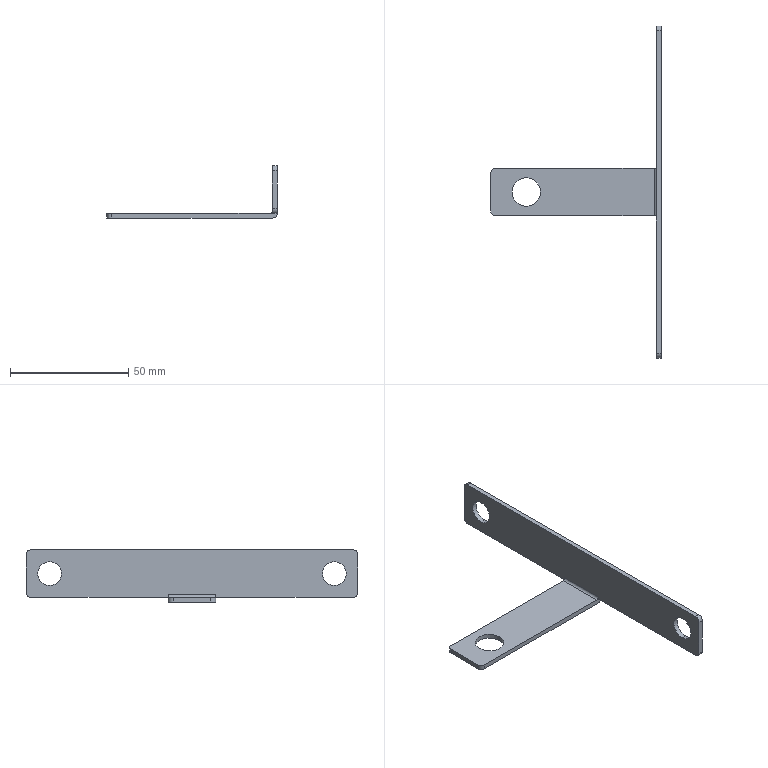Part | SolidWorks | features BaseBody 1 | 1 solid | 26 faces | box 72 x 140.21 x 22 mm | volume 7925 mm3 | cylinder 14 | plane 12 | commonest cylinder face diameters 4 x7 10 x4 12 x2 2 x1
STEP:
#1=CARTESIAN_POINT('',(0.,-10.,-9.));
#2=VERTEX_POINT('',#1);
#3=CARTESIAN_POINT('',(-1.,-10.,-10.));
#4=VERTEX_POINT('',#3);
#5=CARTESIAN_POINT('',(-1.,-10.,-9.));
#6=DIRECTION('',(0.,1.,0.));
#7=DIRECTION('',(0.,0.,1.));
#8=AXIS2_PLACEMENT_3D('',#5,#6,#7);
#9=CIRCLE('',#8,1.);
#10=EDGE_CURVE('',#2,#4,#9,.T.);
#11=ORIENTED_EDGE('',*,*,#10,.F.);
#12=CARTESIAN_POINT('',(0.,10.,-9.));
#13=VERTEX_POINT('',#12);
#14=CARTESIAN_POINT('',(0.,-10.,-9.));
#15=DIRECTION('',(0.,-1.,0.));
#16=VECTOR('',#15,1000.);
#17=LINE('',#14,#16);
#18=EDGE_CURVE('',#13,#2,#17,.T.);
#19=ORIENTED_EDGE('',*,*,#18,.F.);
#20=CARTESIAN_POINT('',(-1.,10.,-10.));
#21=VERTEX_POINT('',#20);
#22=CARTESIAN_POINT('',(-1.,10.,-9.));
#23=DIRECTION('',(0.,-1.,0.));
#24=DIRECTION('',(0.,0.,-1.));
#25=AXIS2_PLACEMENT_3D('',#22,#23,#24);
#26=CIRCLE('',#25,1.);
#27=EDGE_CURVE('',#21,#13,#26,.T.);
#28=ORIENTED_EDGE('',*,*,#27,.F.);
#29=CARTESIAN_POINT('',(-1.,10.,-10.));
#30=DIRECTION('',(0.,1.,0.));
#31=VECTOR('',#30,1000.);
#32=LINE('',#29,#31);
#33=EDGE_CURVE('',#4,#21,#32,.T.);
#34=ORIENTED_EDGE('',*,*,#33,.F.);
#35=EDGE_LOOP('',(#11,#19,#28,#34));
#36=FACE_OUTER_BOUND('',#35,.T.);
#37=CARTESIAN_POINT('',(-1.,8.,-9.));
#38=DIRECTION('',(0.,-1.,0.));
#39=DIRECTION('',(0.,0.,-1.));
#40=AXIS2_PLACEMENT_3D('',#37,#38,#39);
#41=CYLINDRICAL_SURFACE('',#40,1.);
#42=ADVANCED_FACE('',(#36),#41,.F.);
#43=CARTESIAN_POINT('',(2.,10.,-10.));
#44=VERTEX_POINT('',#43);
#45=CARTESIAN_POINT('',(0.,10.,-12.));
#46=VERTEX_POINT('',#45);
#47=CARTESIAN_POINT('',(0.,10.,-10.));
#48=DIRECTION('',(0.,1.,0.));
#49=DIRECTION('',(0.,0.,-1.));
#50=AXIS2_PLACEMENT_3D('',#47,#48,#49);
#51=CIRCLE('',#50,2.);
#52=EDGE_CURVE('',#44,#46,#51,.T.);
#53=ORIENTED_EDGE('',*,*,#52,.F.);
#54=CARTESIAN_POINT('',(2.,-10.,-10.));
#55=VERTEX_POINT('',#54);
#56=CARTESIAN_POINT('',(2.,-68.105,-10.));
#57=DIRECTION('',(0.,1.,0.));
#58=VECTOR('',#57,1000.);
#59=LINE('',#56,#58);
#60=EDGE_CURVE('',#55,#44,#59,.T.);
#61=ORIENTED_EDGE('',*,*,#60,.F.);
#62=CARTESIAN_POINT('',(0.,-10.,-12.));
#63=VERTEX_POINT('',#62);
#64=CARTESIAN_POINT('',(0.,-10.,-10.));
#65=DIRECTION('',(0.,-1.,0.));
#66=DIRECTION('',(0.,0.,1.));
#67=AXIS2_PLACEMENT_3D('',#64,#65,#66);
#68=CIRCLE('',#67,2.);
#69=EDGE_CURVE('',#63,#55,#68,.T.);
#70=ORIENTED_EDGE('',*,*,#69,.F.);
#71=CARTESIAN_POINT('',(0.,8.,-12.));
#72=DIRECTION('',(0.,-1.,0.));
#73=VECTOR('',#72,1000.);
#74=LINE('',#71,#73);
#75=EDGE_CURVE('',#46,#63,#74,.T.);
#76=ORIENTED_EDGE('',*,*,#75,.F.);
#77=EDGE_LOOP('',(#53,#61,#70,#76));
#78=FACE_OUTER_BOUND('',#77,.T.);
#79=CARTESIAN_POINT('',(0.,8.,-10.));
#80=DIRECTION('',(0.,-1.,0.));
#81=DIRECTION('',(0.,0.,-1.));
#82=AXIS2_PLACEMENT_3D('',#79,#80,#81);
#83=CYLINDRICAL_SURFACE('',#82,2.);
#84=ADVANCED_FACE('',(#78),#83,.T.);
#85=CARTESIAN_POINT('',(-61.,0.,-12.));
#86=VERTEX_POINT('',#85);
#87=CARTESIAN_POINT('',(-61.,0.,-10.));
#88=VERTEX_POINT('',#87);
#89=CARTESIAN_POINT('',(-61.,0.,-12.));
#90=DIRECTION('',(0.,0.,1.));
#91=VECTOR('',#90,1000.);
#92=LINE('',#89,#91);
#93=EDGE_CURVE('',#86,#88,#92,.T.);
#94=ORIENTED_EDGE('',*,*,#93,.F.);
#95=CARTESIAN_POINT('',(-49.,0.,-12.));
#96=VERTEX_POINT('',#95);
#97=CARTESIAN_POINT('',(-55.,0.,-12.));
#98=DIRECTION('',(0.,0.,-1.));
#99=DIRECTION('',(-1.,0.,0.));
#100=AXIS2_PLACEMENT_3D('',#97,#98,#99);
#101=CIRCLE('',#100,6.);
#102=EDGE_CURVE('',#86,#96,#101,.T.);
#103=ORIENTED_EDGE('',*,*,#102,.T.);
#104=CARTESIAN_POINT('',(-49.,0.,-10.));
#105=VERTEX_POINT('',#104);
#106=CARTESIAN_POINT('',(-49.,0.,-12.));
#107=DIRECTION('',(0.,0.,1.));
#108=VECTOR('',#107,1000.);
#109=LINE('',#106,#108);
#110=EDGE_CURVE('',#96,#105,#109,.T.);
#111=ORIENTED_EDGE('',*,*,#110,.T.);
#112=CARTESIAN_POINT('',(-55.,0.,-10.));
#113=DIRECTION('',(0.,0.,-1.));
#114=DIRECTION('',(-1.,0.,0.));
#115=AXIS2_PLACEMENT_3D('',#112,#113,#114);
#116=CIRCLE('',#115,6.);
#117=EDGE_CURVE('',#88,#105,#116,.T.);
#118=ORIENTED_EDGE('',*,*,#117,.F.);
#119=EDGE_LOOP('',(#94,#103,#111,#118));
#120=FACE_OUTER_BOUND('',#119,.T.);
#121=CARTESIAN_POINT('',(-55.,0.,-12.));
#122=DIRECTION('',(0.,0.,1.));
#123=DIRECTION('',(1.,0.,0.));
#124=AXIS2_PLACEMENT_3D('',#121,#122,#123);
#125=CYLINDRICAL_SURFACE('',#124,6.);
#126=ADVANCED_FACE('',(#120),#125,.F.);
#127=CARTESIAN_POINT('',(-70.,-8.,-10.));
#128=VERTEX_POINT('',#127);
#129=CARTESIAN_POINT('',(-70.,8.,-10.));
#130=VERTEX_POINT('',#129);
#131=CARTESIAN_POINT('',(-70.,8.,-10.));
#132=DIRECTION('',(0.,1.,0.));
#133=VECTOR('',#132,1000.);
#134=LINE('',#131,#133);
#135=EDGE_CURVE('',#128,#130,#134,.T.);
#136=ORIENTED_EDGE('',*,*,#135,.T.);
#137=CARTESIAN_POINT('',(-70.,8.,-12.));
#138=VERTEX_POINT('',#137);
#139=CARTESIAN_POINT('',(-70.,8.,-12.));
#140=DIRECTION('',(0.,0.,1.));
#141=VECTOR('',#140,1000.);
#142=LINE('',#139,#141);
#143=EDGE_CURVE('',#138,#130,#142,.T.);
#144=ORIENTED_EDGE('',*,*,#143,.F.);
#145=CARTESIAN_POINT('',(-70.,-8.,-12.));
#146=VERTEX_POINT('',#145);
#147=CARTESIAN_POINT('',(-70.,8.,-12.));
#148=DIRECTION('',(0.,1.,0.));
#149=VECTOR('',#148,1000.);
#150=LINE('',#147,#149);
#151=EDGE_CURVE('',#146,#138,#150,.T.);
#152=ORIENTED_EDGE('',*,*,#151,.F.);
#153=CARTESIAN_POINT('',(-70.,-8.,-12.));
#154=DIRECTION('',(0.,0.,1.));
#155=VECTOR('',#154,1000.);
#156=LINE('',#153,#155);
#157=EDGE_CURVE('',#146,#128,#156,.T.);
#158=ORIENTED_EDGE('',*,*,#157,.T.);
#159=EDGE_LOOP('',(#136,#144,#152,#158));
#160=FACE_OUTER_BOUND('',#159,.T.);
#161=CARTESIAN_POINT('',(-70.,8.,-12.));
#162=DIRECTION('',(1.,0.,0.));
#163=DIRECTION('',(0.,1.,0.));
#164=AXIS2_PLACEMENT_3D('',#161,#162,#163);
#165=PLANE('',#164);
#166=ADVANCED_FACE('',(#160),#165,.F.);
#167=CARTESIAN_POINT('',(-68.,-10.,-10.));
#168=VERTEX_POINT('',#167);
#169=CARTESIAN_POINT('',(-68.,-8.,-10.));
#170=DIRECTION('',(0.,0.,-1.));
#171=DIRECTION('',(1.,0.,0.));
#172=AXIS2_PLACEMENT_3D('',#169,#170,#171);
#173=CIRCLE('',#172,2.);
#174=EDGE_CURVE('',#168,#128,#173,.T.);
#175=ORIENTED_EDGE('',*,*,#174,.T.);
#176=ORIENTED_EDGE('',*,*,#157,.F.);
#177=CARTESIAN_POINT('',(-68.,-10.,-12.));
#178=VERTEX_POINT('',#177);
#179=CARTESIAN_POINT('',(-68.,-8.,-12.));
#180=DIRECTION('',(0.,0.,-1.));
#181=DIRECTION('',(1.,0.,0.));
#182=AXIS2_PLACEMENT_3D('',#179,#180,#181);
#183=CIRCLE('',#182,2.);
#184=EDGE_CURVE('',#178,#146,#183,.T.);
#185=ORIENTED_EDGE('',*,*,#184,.F.);
#186=CARTESIAN_POINT('',(-68.,-10.,-12.));
#187=DIRECTION('',(0.,0.,1.));
#188=VECTOR('',#187,1000.);
#189=LINE('',#186,#188);
#190=EDGE_CURVE('',#178,#168,#189,.T.);
#191=ORIENTED_EDGE('',*,*,#190,.T.);
#192=EDGE_LOOP('',(#175,#176,#185,#191));
#193=FACE_OUTER_BOUND('',#192,.T.);
#194=CARTESIAN_POINT('',(-68.,-8.,-12.));
#195=DIRECTION('',(0.,0.,1.));
#196=DIRECTION('',(1.,0.,0.));
#197=AXIS2_PLACEMENT_3D('',#194,#195,#196);
#198=CYLINDRICAL_SURFACE('',#197,2.);
#199=ADVANCED_FACE('',(#193),#198,.T.);
#200=CARTESIAN_POINT('',(-68.,-10.,-12.));
#201=DIRECTION('',(-1.,0.,0.));
#202=VECTOR('',#201,1000.);
#203=LINE('',#200,#202);
#204=EDGE_CURVE('',#63,#178,#203,.T.);
#205=ORIENTED_EDGE('',*,*,#204,.F.);
#206=ORIENTED_EDGE('',*,*,#69,.T.);
#207=CARTESIAN_POINT('',(0.,-10.,-10.));
#208=VERTEX_POINT('',#207);
#209=CARTESIAN_POINT('',(-68.,-10.,-10.));
#210=DIRECTION('',(-1.,0.,0.));
#211=VECTOR('',#210,1000.);
#212=LINE('',#209,#211);
#213=EDGE_CURVE('',#55,#208,#212,.T.);
#214=ORIENTED_EDGE('',*,*,#213,.T.);
#215=CARTESIAN_POINT('',(0.,-10.,-8.));
#216=DIRECTION('',(0.,0.,-1.));
#217=VECTOR('',#216,1000.);
#218=LINE('',#215,#217);
#219=EDGE_CURVE('',#2,#208,#218,.T.);
#220=ORIENTED_EDGE('',*,*,#219,.F.);
#221=ORIENTED_EDGE('',*,*,#10,.T.);
#222=CARTESIAN_POINT('',(-68.,-10.,-10.));
#223=DIRECTION('',(-1.,0.,0.));
#224=VECTOR('',#223,1000.);
#225=LINE('',#222,#224);
#226=EDGE_CURVE('',#4,#168,#225,.T.);
#227=ORIENTED_EDGE('',*,*,#226,.T.);
#228=ORIENTED_EDGE('',*,*,#190,.F.);
#229=EDGE_LOOP('',(#205,#206,#214,#220,#221,#227,#228));
#230=FACE_OUTER_BOUND('',#229,.T.);
#231=CARTESIAN_POINT('',(-68.,-10.,-12.));
#232=DIRECTION('',(0.,1.,0.));
#233=DIRECTION('',(1.,0.,0.));
#234=AXIS2_PLACEMENT_3D('',#231,#232,#233);
#235=PLANE('',#234);
#236=ADVANCED_FACE('',(#230),#235,.F.);
#237=CARTESIAN_POINT('',(0.,10.,-10.));
#238=VERTEX_POINT('',#237);
#239=CARTESIAN_POINT('',(2.,10.,-10.));
#240=DIRECTION('',(1.,0.,0.));
#241=VECTOR('',#240,1000.);
#242=LINE('',#239,#241);
#243=EDGE_CURVE('',#238,#44,#242,.T.);
#244=ORIENTED_EDGE('',*,*,#243,.T.);
#245=ORIENTED_EDGE('',*,*,#52,.T.);
#246=CARTESIAN_POINT('',(-68.,10.,-12.));
#247=VERTEX_POINT('',#246);
#248=CARTESIAN_POINT('',(2.,10.,-12.));
#249=DIRECTION('',(1.,0.,0.));
#250=VECTOR('',#249,1000.);
#251=LINE('',#248,#250);
#252=EDGE_CURVE('',#247,#46,#251,.T.);
#253=ORIENTED_EDGE('',*,*,#252,.F.);
#254=CARTESIAN_POINT('',(-68.,10.,-10.));
#255=VERTEX_POINT('',#254);
#256=CARTESIAN_POINT('',(-68.,10.,-12.));
#257=DIRECTION('',(0.,0.,1.));
#258=VECTOR('',#257,1000.);
#259=LINE('',#256,#258);
#260=EDGE_CURVE('',#247,#255,#259,.T.);
#261=ORIENTED_EDGE('',*,*,#260,.T.);
#262=CARTESIAN_POINT('',(2.,10.,-10.));
#263=DIRECTION('',(1.,0.,0.));
#264=VECTOR('',#263,1000.);
#265=LINE('',#262,#264);
#266=EDGE_CURVE('',#255,#21,#265,.T.);
#267=ORIENTED_EDGE('',*,*,#266,.T.);
#268=ORIENTED_EDGE('',*,*,#27,.T.);
#269=CARTESIAN_POINT('',(0.,10.,-8.));
#270=DIRECTION('',(0.,0.,1.));
#271=VECTOR('',#270,1000.);
#272=LINE('',#269,#271);
#273=EDGE_CURVE('',#238,#13,#272,.T.);
#274=ORIENTED_EDGE('',*,*,#273,.F.);
#275=EDGE_LOOP('',(#244,#245,#253,#261,#267,#268,#274));
#276=FACE_OUTER_BOUND('',#275,.T.);
#277=CARTESIAN_POINT('',(2.,10.,-12.));
#278=DIRECTION('',(0.,-1.,0.));
#279=DIRECTION('',(0.,0.,-1.));
#280=AXIS2_PLACEMENT_3D('',#277,#278,#279);
#281=PLANE('',#280);
#282=ADVANCED_FACE('',(#276),#281,.F.);
#283=CARTESIAN_POINT('',(-68.,8.,-10.));
#284=DIRECTION('',(0.,0.,-1.));
#285=DIRECTION('',(1.,0.,0.));
#286=AXIS2_PLACEMENT_3D('',#283,#284,#285);
#287=CIRCLE('',#286,2.);
#288=EDGE_CURVE('',#130,#255,#287,.T.);
#289=ORIENTED_EDGE('',*,*,#288,.T.);
#290=ORIENTED_EDGE('',*,*,#260,.F.);
#291=CARTESIAN_POINT('',(-68.,8.,-12.));
#292=DIRECTION('',(0.,0.,-1.));
#293=DIRECTION('',(1.,0.,0.));
#294=AXIS2_PLACEMENT_3D('',#291,#292,#293);
#295=CIRCLE('',#294,2.);
#296=EDGE_CURVE('',#138,#247,#295,.T.);
#297=ORIENTED_EDGE('',*,*,#296,.F.);
#298=ORIENTED_EDGE('',*,*,#143,.T.);
#299=EDGE_LOOP('',(#289,#290,#297,#298));
#300=FACE_OUTER_BOUND('',#299,.T.);
#301=CARTESIAN_POINT('',(-68.,8.,-12.));
#302=DIRECTION('',(0.,0.,1.));
#303=DIRECTION('',(1.,0.,0.));
#304=AXIS2_PLACEMENT_3D('',#301,#302,#303);
#305=CYLINDRICAL_SURFACE('',#304,2.);
#306=ADVANCED_FACE('',(#300),#305,.T.);
#307=CARTESIAN_POINT('',(-55.,0.,-10.));
#308=DIRECTION('',(0.,0.,-1.));
#309=DIRECTION('',(-1.,0.,0.));
#310=AXIS2_PLACEMENT_3D('',#307,#308,#309);
#311=CIRCLE('',#310,6.);
#312=EDGE_CURVE('',#105,#88,#311,.T.);
#313=ORIENTED_EDGE('',*,*,#312,.T.);
#314=ORIENTED_EDGE('',*,*,#117,.T.);
#315=EDGE_LOOP('',(#313,#314));
#316=FACE_BOUND('',#315,.T.);
#317=ORIENTED_EDGE('',*,*,#226,.F.);
#318=ORIENTED_EDGE('',*,*,#33,.T.);
#319=ORIENTED_EDGE('',*,*,#266,.F.);
#320=ORIENTED_EDGE('',*,*,#288,.F.);
#321=ORIENTED_EDGE('',*,*,#135,.F.);
#322=ORIENTED_EDGE('',*,*,#174,.F.);
#323=EDGE_LOOP('',(#317,#318,#319,#320,#321,#322));
#324=FACE_OUTER_BOUND('',#323,.T.);
#325=CARTESIAN_POINT('',(-68.,8.,-10.));
#326=DIRECTION('',(0.,0.,1.));
#327=DIRECTION('',(1.,0.,0.));
#328=AXIS2_PLACEMENT_3D('',#325,#326,#327);
#329=PLANE('',#328);
#330=ADVANCED_FACE('',(#316,#324),#329,.T.);
#331=CARTESIAN_POINT('',(-55.,0.,-12.));
#332=DIRECTION('',(0.,0.,-1.));
#333=DIRECTION('',(-1.,0.,0.));
#334=AXIS2_PLACEMENT_3D('',#331,#332,#333);
#335=CIRCLE('',#334,6.);
#336=EDGE_CURVE('',#96,#86,#335,.T.);
#337=ORIENTED_EDGE('',*,*,#336,.F.);
#338=ORIENTED_EDGE('',*,*,#102,.F.);
#339=EDGE_LOOP('',(#337,#338));
#340=FACE_BOUND('',#339,.T.);
#341=ORIENTED_EDGE('',*,*,#252,.T.);
#342=ORIENTED_EDGE('',*,*,#75,.T.);
#343=ORIENTED_EDGE('',*,*,#204,.T.);
#344=ORIENTED_EDGE('',*,*,#184,.T.);
#345=ORIENTED_EDGE('',*,*,#151,.T.);
#346=ORIENTED_EDGE('',*,*,#296,.T.);
#347=EDGE_LOOP('',(#341,#342,#343,#344,#345,#346));
#348=FACE_OUTER_BOUND('',#347,.T.);
#349=CARTESIAN_POINT('',(-68.,8.,-12.));
#350=DIRECTION('',(0.,0.,1.));
#351=DIRECTION('',(1.,0.,0.));
#352=AXIS2_PLACEMENT_3D('',#349,#350,#351);
#353=PLANE('',#352);
#354=ADVANCED_FACE('',(#340,#348),#353,.F.);
#355=CARTESIAN_POINT('',(2.,-60.105,-5.));
#356=VERTEX_POINT('',#355);
#357=CARTESIAN_POINT('',(0.,-60.105,-5.));
#358=VERTEX_POINT('',#357);
#359=CARTESIAN_POINT('',(2.,-60.105,-5.));
#360=DIRECTION('',(-1.,0.,0.));
#361=VECTOR('',#360,1000.);
#362=LINE('',#359,#361);
#363=EDGE_CURVE('',#356,#358,#362,.T.);
#364=ORIENTED_EDGE('',*,*,#363,.F.);
#365=CARTESIAN_POINT('',(2.,-60.105,5.));
#366=VERTEX_POINT('',#365);
#367=CARTESIAN_POINT('',(2.,-60.105,0.));
#368=DIRECTION('',(1.,0.,0.));
#369=DIRECTION('',(0.,0.,-1.));
#370=AXIS2_PLACEMENT_3D('',#367,#368,#369);
#371=CIRCLE('',#370,5.);
#372=EDGE_CURVE('',#356,#366,#371,.T.);
#373=ORIENTED_EDGE('',*,*,#372,.T.);
#374=CARTESIAN_POINT('',(0.,-60.105,5.));
#375=VERTEX_POINT('',#374);
#376=CARTESIAN_POINT('',(2.,-60.105,5.));
#377=DIRECTION('',(-1.,0.,0.));
#378=VECTOR('',#377,1000.);
#379=LINE('',#376,#378);
#380=EDGE_CURVE('',#366,#375,#379,.T.);
#381=ORIENTED_EDGE('',*,*,#380,.T.);
#382=CARTESIAN_POINT('',(0.,-60.105,0.));
#383=DIRECTION('',(1.,0.,0.));
#384=DIRECTION('',(0.,0.,-1.));
#385=AXIS2_PLACEMENT_3D('',#382,#383,#384);
#386=CIRCLE('',#385,5.);
#387=EDGE_CURVE('',#358,#375,#386,.T.);
#388=ORIENTED_EDGE('',*,*,#387,.F.);
#389=EDGE_LOOP('',(#364,#373,#381,#388));
#390=FACE_OUTER_BOUND('',#389,.T.);
#391=CARTESIAN_POINT('',(2.,-60.105,0.));
#392=DIRECTION('',(-1.,0.,0.));
#393=DIRECTION('',(0.,0.,1.));
#394=AXIS2_PLACEMENT_3D('',#391,#392,#393);
#395=CYLINDRICAL_SURFACE('',#394,5.);
#396=ADVANCED_FACE('',(#390),#395,.F.);
#397=CARTESIAN_POINT('',(2.,60.105,-5.));
#398=VERTEX_POINT('',#397);
#399=CARTESIAN_POINT('',(0.,60.105,-5.));
#400=VERTEX_POINT('',#399);
#401=CARTESIAN_POINT('',(2.,60.105,-5.));
#402=DIRECTION('',(-1.,0.,0.));
#403=VECTOR('',#402,1000.);
#404=LINE('',#401,#403);
#405=EDGE_CURVE('',#398,#400,#404,.T.);
#406=ORIENTED_EDGE('',*,*,#405,.F.);
#407=CARTESIAN_POINT('',(2.,60.105,5.));
#408=VERTEX_POINT('',#407);
#409=CARTESIAN_POINT('',(2.,60.105,0.));
#410=DIRECTION('',(1.,0.,0.));
#411=DIRECTION('',(0.,0.,-1.));
#412=AXIS2_PLACEMENT_3D('',#409,#410,#411);
#413=CIRCLE('',#412,5.);
#414=EDGE_CURVE('',#398,#408,#413,.T.);
#415=ORIENTED_EDGE('',*,*,#414,.T.);
#416=CARTESIAN_POINT('',(0.,60.105,5.));
#417=VERTEX_POINT('',#416);
#418=CARTESIAN_POINT('',(2.,60.105,5.));
#419=DIRECTION('',(-1.,0.,0.));
#420=VECTOR('',#419,1000.);
#421=LINE('',#418,#420);
#422=EDGE_CURVE('',#408,#417,#421,.T.);
#423=ORIENTED_EDGE('',*,*,#422,.T.);
#424=CARTESIAN_POINT('',(0.,60.105,0.));
#425=DIRECTION('',(1.,0.,0.));
#426=DIRECTION('',(0.,0.,-1.));
#427=AXIS2_PLACEMENT_3D('',#424,#425,#426);
#428=CIRCLE('',#427,5.);
#429=EDGE_CURVE('',#400,#417,#428,.T.);
#430=ORIENTED_EDGE('',*,*,#429,.F.);
#431=EDGE_LOOP('',(#406,#415,#423,#430));
#432=FACE_OUTER_BOUND('',#431,.T.);
#433=CARTESIAN_POINT('',(2.,60.105,0.));
#434=DIRECTION('',(-1.,0.,0.));
#435=DIRECTION('',(0.,0.,1.));
#436=AXIS2_PLACEMENT_3D('',#433,#434,#435);
#437=CYLINDRICAL_SURFACE('',#436,5.);
#438=ADVANCED_FACE('',(#432),#437,.F.);
#439=CARTESIAN_POINT('',(0.,-70.105,8.));
#440=VERTEX_POINT('',#439);
#441=CARTESIAN_POINT('',(0.,-70.105,-8.));
#442=VERTEX_POINT('',#441);
#443=CARTESIAN_POINT('',(0.,-70.105,8.));
#444=DIRECTION('',(0.,0.,-1.));
#445=VECTOR('',#444,1000.);
#446=LINE('',#443,#445);
#447=EDGE_CURVE('',#440,#442,#446,.T.);
#448=ORIENTED_EDGE('',*,*,#447,.T.);
#449=CARTESIAN_POINT('',(2.,-70.105,-8.));
#450=VERTEX_POINT('',#449);
#451=CARTESIAN_POINT('',(2.,-70.105,-8.));
#452=DIRECTION('',(-1.,0.,0.));
#453=VECTOR('',#452,1000.);
#454=LINE('',#451,#453);
#455=EDGE_CURVE('',#450,#442,#454,.T.);
#456=ORIENTED_EDGE('',*,*,#455,.F.);
#457=CARTESIAN_POINT('',(2.,-70.105,8.));
#458=VERTEX_POINT('',#457);
#459=CARTESIAN_POINT('',(2.,-70.105,8.));
#460=DIRECTION('',(0.,0.,-1.));
#461=VECTOR('',#460,1000.);
#462=LINE('',#459,#461);
#463=EDGE_CURVE('',#458,#450,#462,.T.);
#464=ORIENTED_EDGE('',*,*,#463,.F.);
#465=CARTESIAN_POINT('',(2.,-70.105,8.));
#466=DIRECTION('',(-1.,0.,0.));
#467=VECTOR('',#466,1000.);
#468=LINE('',#465,#467);
#469=EDGE_CURVE('',#458,#440,#468,.T.);
#470=ORIENTED_EDGE('',*,*,#469,.T.);
#471=EDGE_LOOP('',(#448,#456,#464,#470));
#472=FACE_OUTER_BOUND('',#471,.T.);
#473=CARTESIAN_POINT('',(2.,-70.105,8.));
#474=DIRECTION('',(0.,1.,0.));
#475=DIRECTION('',(1.,0.,0.));
#476=AXIS2_PLACEMENT_3D('',#473,#474,#475);
#477=PLANE('',#476);
#478=ADVANCED_FACE('',(#472),#477,.F.);
#479=CARTESIAN_POINT('',(0.,-68.105,10.));
#480=VERTEX_POINT('',#479);
#481=CARTESIAN_POINT('',(0.,-68.105,8.));
#482=DIRECTION('',(1.,0.,0.));
#483=DIRECTION('',(0.,0.,-1.));
#484=AXIS2_PLACEMENT_3D('',#481,#482,#483);
#485=CIRCLE('',#484,2.);
#486=EDGE_CURVE('',#480,#440,#485,.T.);
#487=ORIENTED_EDGE('',*,*,#486,.T.);
#488=ORIENTED_EDGE('',*,*,#469,.F.);
#489=CARTESIAN_POINT('',(2.,-68.105,10.));
#490=VERTEX_POINT('',#489);
#491=CARTESIAN_POINT('',(2.,-68.105,8.));
#492=DIRECTION('',(1.,0.,0.));
#493=DIRECTION('',(0.,0.,-1.));
#494=AXIS2_PLACEMENT_3D('',#491,#492,#493);
#495=CIRCLE('',#494,2.);
#496=EDGE_CURVE('',#490,#458,#495,.T.);
#497=ORIENTED_EDGE('',*,*,#496,.F.);
#498=CARTESIAN_POINT('',(2.,-68.105,10.));
#499=DIRECTION('',(-1.,0.,0.));
#500=VECTOR('',#499,1000.);
#501=LINE('',#498,#500);
#502=EDGE_CURVE('',#490,#480,#501,.T.);
#503=ORIENTED_EDGE('',*,*,#502,.T.);
#504=EDGE_LOOP('',(#487,#488,#497,#503));
#505=FACE_OUTER_BOUND('',#504,.T.);
#506=CARTESIAN_POINT('',(2.,-68.105,8.));
#507=DIRECTION('',(-1.,0.,0.));
#508=DIRECTION('',(0.,0.,1.));
#509=AXIS2_PLACEMENT_3D('',#506,#507,#508);
#510=CYLINDRICAL_SURFACE('',#509,2.);
#511=ADVANCED_FACE('',(#505),#510,.T.);
#512=CARTESIAN_POINT('',(0.,68.105,10.));
#513=VERTEX_POINT('',#512);
#514=CARTESIAN_POINT('',(0.,68.105,10.));
#515=DIRECTION('',(0.,-1.,0.));
#516=VECTOR('',#515,1000.);
#517=LINE('',#514,#516);
#518=EDGE_CURVE('',#513,#480,#517,.T.);
#519=ORIENTED_EDGE('',*,*,#518,.T.);
#520=ORIENTED_EDGE('',*,*,#502,.F.);
#521=CARTESIAN_POINT('',(2.,68.105,10.));
#522=VERTEX_POINT('',#521);
#523=CARTESIAN_POINT('',(2.,68.105,10.));
#524=DIRECTION('',(0.,-1.,0.));
#525=VECTOR('',#524,1000.);
#526=LINE('',#523,#525);
#527=EDGE_CURVE('',#522,#490,#526,.T.);
#528=ORIENTED_EDGE('',*,*,#527,.F.);
#529=CARTESIAN_POINT('',(2.,68.105,10.));
#530=DIRECTION('',(-1.,0.,0.));
#531=VECTOR('',#530,1000.);
#532=LINE('',#529,#531);
#533=EDGE_CURVE('',#522,#513,#532,.T.);
#534=ORIENTED_EDGE('',*,*,#533,.T.);
#535=EDGE_LOOP('',(#519,#520,#528,#534));
#536=FACE_OUTER_BOUND('',#535,.T.);
#537=CARTESIAN_POINT('',(2.,68.105,10.));
#538=DIRECTION('',(0.,0.,-1.));
#539=DIRECTION('',(0.,-1.,0.));
#540=AXIS2_PLACEMENT_3D('',#537,#538,#539);
#541=PLANE('',#540);
#542=ADVANCED_FACE('',(#536),#541,.F.);
#543=CARTESIAN_POINT('',(0.,70.105,8.));
#544=VERTEX_POINT('',#543);
#545=CARTESIAN_POINT('',(0.,68.105,8.));
#546=DIRECTION('',(1.,0.,0.));
#547=DIRECTION('',(0.,0.,1.));
#548=AXIS2_PLACEMENT_3D('',#545,#546,#547);
#549=CIRCLE('',#548,2.);
#550=EDGE_CURVE('',#544,#513,#549,.T.);
#551=ORIENTED_EDGE('',*,*,#550,.T.);
#552=ORIENTED_EDGE('',*,*,#533,.F.);
#553=CARTESIAN_POINT('',(2.,70.105,8.));
#554=VERTEX_POINT('',#553);
#555=CARTESIAN_POINT('',(2.,68.105,8.));
#556=DIRECTION('',(1.,0.,0.));
#557=DIRECTION('',(0.,0.,1.));
#558=AXIS2_PLACEMENT_3D('',#555,#556,#557);
#559=CIRCLE('',#558,2.);
#560=EDGE_CURVE('',#554,#522,#559,.T.);
#561=ORIENTED_EDGE('',*,*,#560,.F.);
#562=CARTESIAN_POINT('',(2.,70.105,8.));
#563=DIRECTION('',(-1.,0.,0.));
#564=VECTOR('',#563,1000.);
#565=LINE('',#562,#564);
#566=EDGE_CURVE('',#554,#544,#565,.T.);
#567=ORIENTED_EDGE('',*,*,#566,.T.);
#568=EDGE_LOOP('',(#551,#552,#561,#567));
#569=FACE_OUTER_BOUND('',#568,.T.);
#570=CARTESIAN_POINT('',(2.,68.105,8.));
#571=DIRECTION('',(-1.,0.,0.));
#572=DIRECTION('',(0.,0.,1.));
#573=AXIS2_PLACEMENT_3D('',#570,#571,#572);
#574=CYLINDRICAL_SURFACE('',#573,2.);
#575=ADVANCED_FACE('',(#569),#574,.T.);
#576=CARTESIAN_POINT('',(0.,70.105,-8.));
#577=VERTEX_POINT('',#576);
#578=CARTESIAN_POINT('',(0.,70.105,8.));
#579=DIRECTION('',(0.,0.,1.));
#580=VECTOR('',#579,1000.);
#581=LINE('',#578,#580);
#582=EDGE_CURVE('',#577,#544,#581,.T.);
#583=ORIENTED_EDGE('',*,*,#582,.T.);
#584=ORIENTED_EDGE('',*,*,#566,.F.);
#585=CARTESIAN_POINT('',(2.,70.105,-8.));
#586=VERTEX_POINT('',#585);
#587=CARTESIAN_POINT('',(2.,70.105,8.));
#588=DIRECTION('',(0.,0.,1.));
#589=VECTOR('',#588,1000.);
#590=LINE('',#587,#589);
#591=EDGE_CURVE('',#586,#554,#590,.T.);
#592=ORIENTED_EDGE('',*,*,#591,.F.);
#593=CARTESIAN_POINT('',(2.,70.105,-8.));
#594=DIRECTION('',(-1.,0.,0.));
#595=VECTOR('',#594,1000.);
#596=LINE('',#593,#595);
#597=EDGE_CURVE('',#586,#577,#596,.T.);
#598=ORIENTED_EDGE('',*,*,#597,.T.);
#599=EDGE_LOOP('',(#583,#584,#592,#598));
#600=FACE_OUTER_BOUND('',#599,.T.);
#601=CARTESIAN_POINT('',(2.,70.105,8.));
#602=DIRECTION('',(0.,-1.,0.));
#603=DIRECTION('',(0.,0.,-1.));
#604=AXIS2_PLACEMENT_3D('',#601,#602,#603);
#605=PLANE('',#604);
#606=ADVANCED_FACE('',(#600),#605,.F.);
#607=CARTESIAN_POINT('',(0.,68.105,-10.));
#608=VERTEX_POINT('',#607);
#609=CARTESIAN_POINT('',(0.,68.105,-8.));
#610=DIRECTION('',(1.,0.,0.));
#611=DIRECTION('',(0.,0.,-1.));
#612=AXIS2_PLACEMENT_3D('',#609,#610,#611);
#613=CIRCLE('',#612,2.);
#614=EDGE_CURVE('',#608,#577,#613,.T.);
#615=ORIENTED_EDGE('',*,*,#614,.T.);
#616=ORIENTED_EDGE('',*,*,#597,.F.);
#617=CARTESIAN_POINT('',(2.,68.105,-10.));
#618=VERTEX_POINT('',#617);
#619=CARTESIAN_POINT('',(2.,68.105,-8.));
#620=DIRECTION('',(1.,0.,0.));
#621=DIRECTION('',(0.,0.,-1.));
#622=AXIS2_PLACEMENT_3D('',#619,#620,#621);
#623=CIRCLE('',#622,2.);
#624=EDGE_CURVE('',#618,#586,#623,.T.);
#625=ORIENTED_EDGE('',*,*,#624,.F.);
#626=CARTESIAN_POINT('',(2.,68.105,-10.));
#627=DIRECTION('',(-1.,0.,0.));
#628=VECTOR('',#627,1000.);
#629=LINE('',#626,#628);
#630=EDGE_CURVE('',#618,#608,#629,.T.);
#631=ORIENTED_EDGE('',*,*,#630,.T.);
#632=EDGE_LOOP('',(#615,#616,#625,#631));
#633=FACE_OUTER_BOUND('',#632,.T.);
#634=CARTESIAN_POINT('',(2.,68.105,-8.));
#635=DIRECTION('',(-1.,0.,0.));
#636=DIRECTION('',(0.,0.,1.));
#637=AXIS2_PLACEMENT_3D('',#634,#635,#636);
#638=CYLINDRICAL_SURFACE('',#637,2.);
#639=ADVANCED_FACE('',(#633),#638,.T.);
#640=CARTESIAN_POINT('',(0.,-68.105,-10.));
#641=VERTEX_POINT('',#640);
#642=CARTESIAN_POINT('',(0.,-68.105,-8.));
#643=DIRECTION('',(1.,0.,0.));
#644=DIRECTION('',(0.,0.,1.));
#645=AXIS2_PLACEMENT_3D('',#642,#643,#644);
#646=CIRCLE('',#645,2.);
#647=EDGE_CURVE('',#442,#641,#646,.T.);
#648=ORIENTED_EDGE('',*,*,#647,.T.);
#649=CARTESIAN_POINT('',(2.,-68.105,-10.));
#650=VERTEX_POINT('',#649);
#651=CARTESIAN_POINT('',(2.,-68.105,-10.));
#652=DIRECTION('',(-1.,0.,0.));
#653=VECTOR('',#652,1000.);
#654=LINE('',#651,#653);
#655=EDGE_CURVE('',#650,#641,#654,.T.);
#656=ORIENTED_EDGE('',*,*,#655,.F.);
#657=CARTESIAN_POINT('',(2.,-68.105,-8.));
#658=DIRECTION('',(1.,0.,0.));
#659=DIRECTION('',(0.,0.,1.));
#660=AXIS2_PLACEMENT_3D('',#657,#658,#659);
#661=CIRCLE('',#660,2.);
#662=EDGE_CURVE('',#450,#650,#661,.T.);
#663=ORIENTED_EDGE('',*,*,#662,.F.);
#664=ORIENTED_EDGE('',*,*,#455,.T.);
#665=EDGE_LOOP('',(#648,#656,#663,#664));
#666=FACE_OUTER_BOUND('',#665,.T.);
#667=CARTESIAN_POINT('',(2.,-68.105,-8.));
#668=DIRECTION('',(-1.,0.,0.));
#669=DIRECTION('',(0.,0.,1.));
#670=AXIS2_PLACEMENT_3D('',#667,#668,#669);
#671=CYLINDRICAL_SURFACE('',#670,2.);
#672=ADVANCED_FACE('',(#666),#671,.T.);
#673=CARTESIAN_POINT('',(0.,-60.105,0.));
#674=DIRECTION('',(1.,0.,0.));
#675=DIRECTION('',(0.,0.,-1.));
#676=AXIS2_PLACEMENT_3D('',#673,#674,#675);
#677=CIRCLE('',#676,5.);
#678=EDGE_CURVE('',#375,#358,#677,.T.);
#679=ORIENTED_EDGE('',*,*,#678,.T.);
#680=ORIENTED_EDGE('',*,*,#387,.T.);
#681=EDGE_LOOP('',(#679,#680));
#682=FACE_BOUND('',#681,.T.);
#683=CARTESIAN_POINT('',(0.,60.105,0.));
#684=DIRECTION('',(1.,0.,0.));
#685=DIRECTION('',(0.,0.,-1.));
#686=AXIS2_PLACEMENT_3D('',#683,#684,#685);
#687=CIRCLE('',#686,5.);
#688=EDGE_CURVE('',#417,#400,#687,.T.);
#689=ORIENTED_EDGE('',*,*,#688,.T.);
#690=ORIENTED_EDGE('',*,*,#429,.T.);
#691=EDGE_LOOP('',(#689,#690));
#692=FACE_BOUND('',#691,.T.);
#693=CARTESIAN_POINT('',(0.,68.105,-10.));
#694=DIRECTION('',(0.,1.,0.));
#695=VECTOR('',#694,1000.);
#696=LINE('',#693,#695);
#697=EDGE_CURVE('',#238,#608,#696,.T.);
#698=ORIENTED_EDGE('',*,*,#697,.F.);
#699=ORIENTED_EDGE('',*,*,#273,.T.);
#700=ORIENTED_EDGE('',*,*,#18,.T.);
#701=ORIENTED_EDGE('',*,*,#219,.T.);
#702=CARTESIAN_POINT('',(0.,68.105,-10.));
#703=DIRECTION('',(0.,1.,0.));
#704=VECTOR('',#703,1000.);
#705=LINE('',#702,#704);
#706=EDGE_CURVE('',#641,#208,#705,.T.);
#707=ORIENTED_EDGE('',*,*,#706,.F.);
#708=ORIENTED_EDGE('',*,*,#647,.F.);
#709=ORIENTED_EDGE('',*,*,#447,.F.);
#710=ORIENTED_EDGE('',*,*,#486,.F.);
#711=ORIENTED_EDGE('',*,*,#518,.F.);
#712=ORIENTED_EDGE('',*,*,#550,.F.);
#713=ORIENTED_EDGE('',*,*,#582,.F.);
#714=ORIENTED_EDGE('',*,*,#614,.F.);
#715=EDGE_LOOP('',(#698,#699,#700,#701,#707,#708,#709,#710,#711,#712,#713,#714));
#716=FACE_OUTER_BOUND('',#715,.T.);
#717=CARTESIAN_POINT('',(0.,-68.105,-8.));
#718=DIRECTION('',(-1.,0.,0.));
#719=DIRECTION('',(0.,0.,1.));
#720=AXIS2_PLACEMENT_3D('',#717,#718,#719);
#721=PLANE('',#720);
#722=ADVANCED_FACE('',(#682,#692,#716),#721,.T.);
#723=CARTESIAN_POINT('',(2.,-60.105,0.));
#724=DIRECTION('',(1.,0.,0.));
#725=DIRECTION('',(0.,0.,-1.));
#726=AXIS2_PLACEMENT_3D('',#723,#724,#725);
#727=CIRCLE('',#726,5.);
#728=EDGE_CURVE('',#366,#356,#727,.T.);
#729=ORIENTED_EDGE('',*,*,#728,.F.);
#730=ORIENTED_EDGE('',*,*,#372,.F.);
#731=EDGE_LOOP('',(#729,#730));
#732=FACE_BOUND('',#731,.T.);
#733=CARTESIAN_POINT('',(2.,60.105,0.));
#734=DIRECTION('',(1.,0.,0.));
#735=DIRECTION('',(0.,0.,-1.));
#736=AXIS2_PLACEMENT_3D('',#733,#734,#735);
#737=CIRCLE('',#736,5.);
#738=EDGE_CURVE('',#408,#398,#737,.T.);
#739=ORIENTED_EDGE('',*,*,#738,.F.);
#740=ORIENTED_EDGE('',*,*,#414,.F.);
#741=EDGE_LOOP('',(#739,#740));
#742=FACE_BOUND('',#741,.T.);
#743=CARTESIAN_POINT('',(2.,68.105,-10.));
#744=DIRECTION('',(0.,1.,0.));
#745=VECTOR('',#744,1000.);
#746=LINE('',#743,#745);
#747=EDGE_CURVE('',#650,#55,#746,.T.);
#748=ORIENTED_EDGE('',*,*,#747,.T.);
#749=ORIENTED_EDGE('',*,*,#60,.T.);
#750=CARTESIAN_POINT('',(2.,68.105,-10.));
#751=DIRECTION('',(0.,1.,0.));
#752=VECTOR('',#751,1000.);
#753=LINE('',#750,#752);
#754=EDGE_CURVE('',#44,#618,#753,.T.);
#755=ORIENTED_EDGE('',*,*,#754,.T.);
#756=ORIENTED_EDGE('',*,*,#624,.T.);
#757=ORIENTED_EDGE('',*,*,#591,.T.);
#758=ORIENTED_EDGE('',*,*,#560,.T.);
#759=ORIENTED_EDGE('',*,*,#527,.T.);
#760=ORIENTED_EDGE('',*,*,#496,.T.);
#761=ORIENTED_EDGE('',*,*,#463,.T.);
#762=ORIENTED_EDGE('',*,*,#662,.T.);
#763=EDGE_LOOP('',(#748,#749,#755,#756,#757,#758,#759,#760,#761,#762));
#764=FACE_OUTER_BOUND('',#763,.T.);
#765=CARTESIAN_POINT('',(2.,-68.105,-8.));
#766=DIRECTION('',(-1.,0.,0.));
#767=DIRECTION('',(0.,0.,1.));
#768=AXIS2_PLACEMENT_3D('',#765,#766,#767);
#769=PLANE('',#768);
#770=ADVANCED_FACE('',(#732,#742,#764),#769,.F.);
#771=ORIENTED_EDGE('',*,*,#213,.F.);
#772=ORIENTED_EDGE('',*,*,#747,.F.);
#773=ORIENTED_EDGE('',*,*,#655,.T.);
#774=ORIENTED_EDGE('',*,*,#706,.T.);
#775=EDGE_LOOP('',(#771,#772,#773,#774));
#776=FACE_OUTER_BOUND('',#775,.T.);
#777=CARTESIAN_POINT('',(2.,68.105,-10.));
#778=DIRECTION('',(0.,0.,1.));
#779=DIRECTION('',(1.,0.,0.));
#780=AXIS2_PLACEMENT_3D('',#777,#778,#779);
#781=PLANE('',#780);
#782=ADVANCED_FACE('',(#776),#781,.F.);
#783=ORIENTED_EDGE('',*,*,#243,.F.);
#784=ORIENTED_EDGE('',*,*,#697,.T.);
#785=ORIENTED_EDGE('',*,*,#630,.F.);
#786=ORIENTED_EDGE('',*,*,#754,.F.);
#787=EDGE_LOOP('',(#783,#784,#785,#786));
#788=FACE_OUTER_BOUND('',#787,.T.);
#789=CARTESIAN_POINT('',(2.,68.105,-10.));
#790=DIRECTION('',(0.,0.,1.));
#791=DIRECTION('',(1.,0.,0.));
#792=AXIS2_PLACEMENT_3D('',#789,#790,#791);
#793=PLANE('',#792);
#794=ADVANCED_FACE('',(#788),#793,.F.);
#795=ORIENTED_EDGE('',*,*,#738,.T.);
#796=ORIENTED_EDGE('',*,*,#405,.T.);
#797=ORIENTED_EDGE('',*,*,#688,.F.);
#798=ORIENTED_EDGE('',*,*,#422,.F.);
#799=EDGE_LOOP('',(#795,#796,#797,#798));
#800=FACE_OUTER_BOUND('',#799,.T.);
#801=CARTESIAN_POINT('',(2.,60.105,0.));
#802=DIRECTION('',(-1.,0.,0.));
#803=DIRECTION('',(0.,0.,1.));
#804=AXIS2_PLACEMENT_3D('',#801,#802,#803);
#805=CYLINDRICAL_SURFACE('',#804,5.);
#806=ADVANCED_FACE('',(#800),#805,.F.);
#807=ORIENTED_EDGE('',*,*,#728,.T.);
#808=ORIENTED_EDGE('',*,*,#363,.T.);
#809=ORIENTED_EDGE('',*,*,#678,.F.);
#810=ORIENTED_EDGE('',*,*,#380,.F.);
#811=EDGE_LOOP('',(#807,#808,#809,#810));
#812=FACE_OUTER_BOUND('',#811,.T.);
#813=CARTESIAN_POINT('',(2.,-60.105,0.));
#814=DIRECTION('',(-1.,0.,0.));
#815=DIRECTION('',(0.,0.,1.));
#816=AXIS2_PLACEMENT_3D('',#813,#814,#815);
#817=CYLINDRICAL_SURFACE('',#816,5.);
#818=ADVANCED_FACE('',(#812),#817,.F.);
#819=ORIENTED_EDGE('',*,*,#336,.T.);
#820=ORIENTED_EDGE('',*,*,#93,.T.);
#821=ORIENTED_EDGE('',*,*,#312,.F.);
#822=ORIENTED_EDGE('',*,*,#110,.F.);
#823=EDGE_LOOP('',(#819,#820,#821,#822));
#824=FACE_OUTER_BOUND('',#823,.T.);
#825=CARTESIAN_POINT('',(-55.,0.,-12.));
#826=DIRECTION('',(0.,0.,1.));
#827=DIRECTION('',(1.,0.,0.));
#828=AXIS2_PLACEMENT_3D('',#825,#826,#827);
#829=CYLINDRICAL_SURFACE('',#828,6.);
#830=ADVANCED_FACE('',(#824),#829,.F.);
#831=CLOSED_SHELL('',(#42,#84,#126,#166,#199,#236,#282,#306,#330,#354,#396,#438,#478,#511,#542,#575,#606,#639,#672,#722,#770,#782,#794,#806,#818,#830));
#832=MANIFOLD_SOLID_BREP('',#831);
#833=CARTESIAN_POINT('',(0.,0.,0.));
#834=DIRECTION('',(0.,0.,1.));
#835=DIRECTION('',(1.,0.,0.));
#836=AXIS2_PLACEMENT_3D('',#833,#834,#835);
#837=(LENGTH_UNIT()NAMED_UNIT(*)SI_UNIT(.MILLI.,.METRE.));
#838=UNCERTAINTY_MEASURE_WITH_UNIT(LENGTH_MEASURE(0.00001),#837,'','');
#839=(NAMED_UNIT(*)PLANE_ANGLE_UNIT()SI_UNIT($,.RADIAN.));
#840=(NAMED_UNIT(*)SI_UNIT($,.STERADIAN.)SOLID_ANGLE_UNIT());
#841=(GEOMETRIC_REPRESENTATION_CONTEXT(3)GLOBAL_UNCERTAINTY_ASSIGNED_CONTEXT((#838))GLOBAL_UNIT_ASSIGNED_CONTEXT((#837,#839,#840))REPRESENTATION_CONTEXT('',''));
#842=ADVANCED_BREP_SHAPE_REPRESENTATION('',(#832,#836),#841);